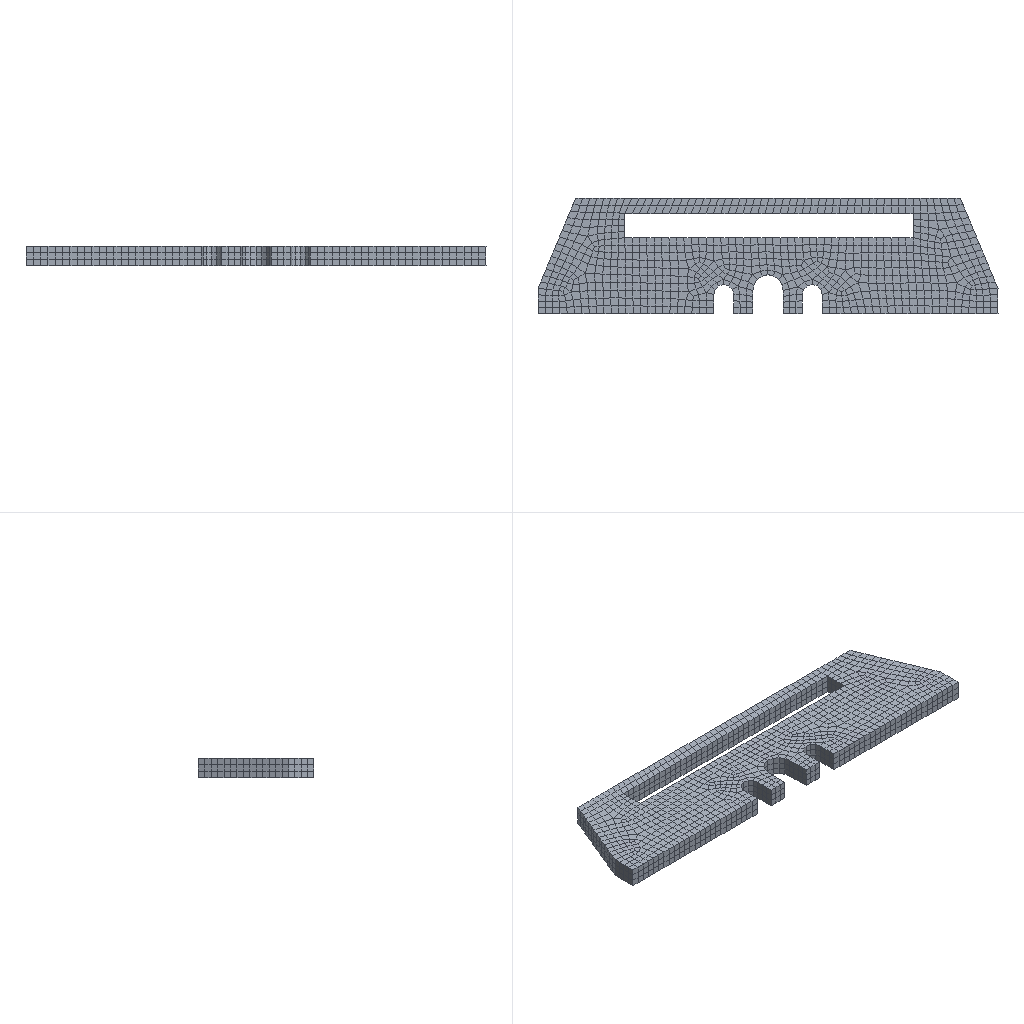Simulation study | ansys workbench
Set-up summary:
category,name,step,type,value,unit,region
solver,ansys_workbench
units,mm-N-s-tonne (MPa),,stated,"/units,MPA"
analysis,deck-1/LS1,,steady-state thermal
load_step,deck-1/LS1,deck-1/LS1,steady-state thermal,nsubst=1; time=1
analysis,deck-2/LS1,,static
load_step,deck-2/LS1,deck-2/LS1,static,nsubst=1; time=1
mesh,deck-1.dat,,nodes,13515
mesh,deck-1.dat,,elements,3054
element_type,SOLID90,,,2406,,deck-1.dat
element_type,SURF152,,,648,,deck-1.dat
mesh,deck-2.dat,,nodes,13515
mesh,deck-2.dat,,elements,3208
element_type,SOLID186,,,2406,,deck-2.dat
element_type,SURF154,,,802,,deck-2.dat
material,wall,,E,2230,tonne s^-2 mm^-1
material,wall,,nu,0.1
material,wall,,density,1.64e-09,tonne mm^-3
material,wall,,conductivity,52.78,tonne mm s^-3 C^-1
material,wall,,specific_heat,9.6e+08,mm^2 s^-2 C^-1
material,wall,,cte,5e-06,C^-1
load,Define Uniform Initial temperature,deck-1/model,body load temp,5,,all
load,"Create ""Convection""",deck-1/LS1,convection,0.005,,SURF152 #2
load,Define Pressure Using Surface Effect Elements,deck-2/LS1,pressure,0.025,,SURF154 #2
load,"Create Imported Load ""Imported Body Temperature""",deck-2/LS1,body load temp,-15 [n=13515],,all
bc,,deck-1/LS1,temperature,-15 [dofs=TEMP],,node list
bc,Constant Zero Displacement X,deck-2/model,fixed,[dofs=UX],,_DISPZEROUX
bc,Constant Zero Displacement Y,deck-2/model,fixed,[dofs=UY],,_DISPZEROUY
bc,Constant Zero Displacement Z,deck-2/model,fixed,[dofs=UZ],,_DISPZEROUZ
named_set,_CM29,,node,2676
named_set,_DISPZEROUX,,node,622
named_set,_DISPZEROUY,,node,622
named_set,_DISPZEROUZ,,node,622
Results summary:
result,analyses[0].index,,,1
result,analyses[0].system,,,SYS-5
result,analyses[0].deck,,,deck-1.dat
result,analyses[0].solve_status,,,completed
result,analyses[0].analysis_type,,,static
result,analyses[0].physics,,,thermal
result,analyses[0].unit_system,,,"NMM: mm, ton, N, s, mV, mA, degC"
result,analyses[0].n_sets,,,1
result,analyses[0].load_steps[0].set,set=1,,1
result,analyses[0].load_steps[0].time_or_freq,set=1,,1
result,analyses[0].load_steps[0].max_temperature,set=1,,-8.97
result,analyses[0].load_steps[0].min_temperature,set=1,,-15
result,analyses[1].index,,,2
result,analyses[1].system,,,SYS-6
result,analyses[1].deck,,,deck-2.dat
result,analyses[1].solve_status,,,completed
result,analyses[1].analysis_type,,,static
result,analyses[1].physics,,,mechanical
result,analyses[1].unit_system,,,"NMM: mm, ton, N, s, mV, mA, degC"
result,analyses[1].n_sets,,,1
result,analyses[1].load_steps[0].set,set=1,,1
result,analyses[1].load_steps[0].time_or_freq,set=1,,1
result,analyses[1].load_steps[0].max_displacement_magnitude,set=1,,100.128
result,analyses[1].load_steps[0].max_von_mises_nodal,set=1,,3.369
result,analyses[1].load_steps[0].reaction_force_sum_xyz[1],set=1,,0.01913
result,analyses[1].load_steps[0].reaction_force_sum_xyz[2],set=1,,-0.2637
result,analyses[1].load_steps[0].reaction_force_sum_xyz[3],set=1,,7.38137e+06
result,geometry_export[0][0],,,.step
result,geometry_export[0][1],,,ok
result,geometry_export[0][2],,,1